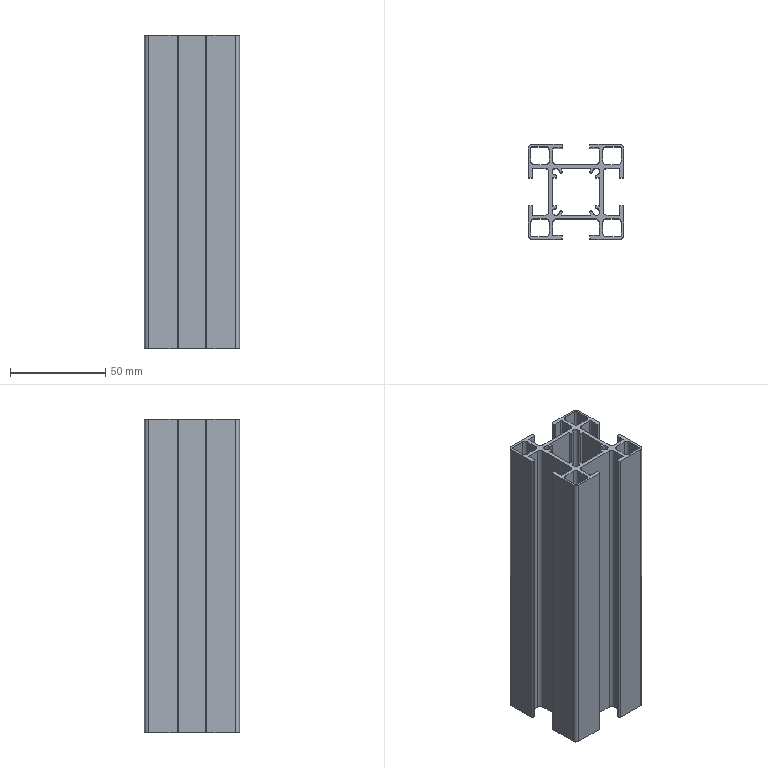Part | STEP file | 46A-00006CC11-165mm | 1 solid | 142 faces | box 50 x 50 x 165 mm | volume 96936 mm3 | cylinder 84 | plane 58 | commonest cylinder face diameters 1 x24 4 x24 1.5 x16 3.7 x8 6.7 x8 2 x4